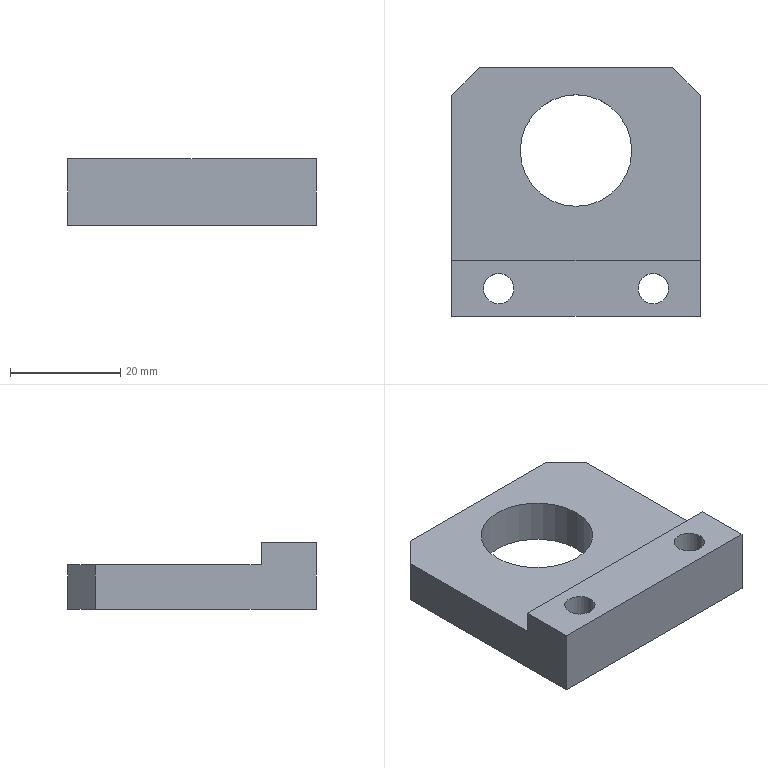Part | STEP file | detection cylinder seat--1 | 1 solid | 16 faces | box 45 x 45 x 12 mm | volume 14666 mm3 | plane 10 | cylinder 6 | commonest cylinder face diameters 5.5 x4 20.2 x2
STEP:
#1=CARTESIAN_POINT('',(0.,0.,0.));
#2=DIRECTION('',(0.,0.,1.));
#3=DIRECTION('',(1.,0.,0.));
#4=AXIS2_PLACEMENT_3D('',#1,#2,#3);
#5=CARTESIAN_POINT('',(11.25,-25.,12.));
#6=VERTEX_POINT('',#5);
#7=CARTESIAN_POINT('',(11.25,-25.,0.));
#8=VERTEX_POINT('',#7);
#9=CARTESIAN_POINT('',(11.25,-25.,12.));
#10=DIRECTION('',(0.,0.,-1.));
#11=VECTOR('',#10,1.);
#12=LINE('',#9,#11);
#13=CARTESIAN_POINT('',(14.,-25.,12.));
#14=DIRECTION('',(0.,0.,-1.));
#15=DIRECTION('',(-1.,0.,0.));
#16=AXIS2_PLACEMENT_3D('',#13,#14,#15);
#17=CYLINDRICAL_SURFACE('',#16,2.75);
#18=CARTESIAN_POINT('',(6.283,0.));
#19=DIRECTION('',(0.,1.));
#20=VECTOR('',#19,1.);
#21=LINE('',#18,#20);
#22=(GEOMETRIC_REPRESENTATION_CONTEXT(2)PARAMETRIC_REPRESENTATION_CONTEXT()REPRESENTATION_CONTEXT('',''));
#23=DEFINITIONAL_REPRESENTATION('',(#21),#22);
#24=PCURVE('',#17,#23);
#25=CARTESIAN_POINT('',(14.,-25.,12.));
#26=DIRECTION('',(0.,0.,-1.));
#27=DIRECTION('',(-1.,0.,0.));
#28=AXIS2_PLACEMENT_3D('',#25,#26,#27);
#29=CYLINDRICAL_SURFACE('',#28,2.75);
#30=CARTESIAN_POINT('',(0.,0.));
#31=DIRECTION('',(0.,1.));
#32=VECTOR('',#31,1.);
#33=LINE('',#30,#32);
#34=(GEOMETRIC_REPRESENTATION_CONTEXT(2)PARAMETRIC_REPRESENTATION_CONTEXT()REPRESENTATION_CONTEXT('',''));
#35=DEFINITIONAL_REPRESENTATION('',(#33),#34);
#36=PCURVE('',#29,#35);
#37=SURFACE_CURVE('',#12,(#24,#36),.PCURVE_S1.);
#38=EDGE_CURVE('',#6,#8,#37,.T.);
#39=ORIENTED_EDGE('',*,*,#38,.T.);
#40=CARTESIAN_POINT('',(16.75,-25.,0.));
#41=VERTEX_POINT('',#40);
#42=CARTESIAN_POINT('',(14.,-25.,0.));
#43=DIRECTION('',(0.,0.,-1.));
#44=DIRECTION('',(-1.,0.,0.));
#45=AXIS2_PLACEMENT_3D('',#42,#43,#44);
#46=CIRCLE('',#45,2.75);
#47=CARTESIAN_POINT('',(0.,12.));
#48=DIRECTION('',(1.,0.));
#49=VECTOR('',#48,1.);
#50=LINE('',#47,#49);
#51=(GEOMETRIC_REPRESENTATION_CONTEXT(2)PARAMETRIC_REPRESENTATION_CONTEXT()REPRESENTATION_CONTEXT('',''));
#52=DEFINITIONAL_REPRESENTATION('',(#50),#51);
#53=PCURVE('',#17,#52);
#54=CARTESIAN_POINT('',(-22.5,-30.,0.));
#55=DIRECTION('',(0.,0.,1.));
#56=DIRECTION('',(1.,0.,0.));
#57=AXIS2_PLACEMENT_3D('',#54,#55,#56);
#58=PLANE('',#57);
#59=CARTESIAN_POINT('',(33.75,5.));
#60=CARTESIAN_POINT('',(33.75,9.763));
#61=CARTESIAN_POINT('',(37.875,7.382));
#62=CARTESIAN_POINT('',(42.,5.));
#63=CARTESIAN_POINT('',(37.875,2.618));
#64=CARTESIAN_POINT('',(33.75,0.2369));
#65=CARTESIAN_POINT('',(33.75,5.));
#66=(BOUNDED_CURVE()B_SPLINE_CURVE(2,(#59,#60,#61,#62,#63,#64,#65),.UNSPECIFIED.,.T.,.F.)B_SPLINE_CURVE_WITH_KNOTS((1,2,2,2,2,1),(-2.094,0.,2.094,4.189,6.283,8.378),.UNSPECIFIED.)CURVE()GEOMETRIC_REPRESENTATION_ITEM()RATIONAL_B_SPLINE_CURVE((1.,0.5,1.,0.5,1.,0.5,1.))REPRESENTATION_ITEM(''));
#67=(GEOMETRIC_REPRESENTATION_CONTEXT(2)PARAMETRIC_REPRESENTATION_CONTEXT()REPRESENTATION_CONTEXT('',''));
#68=DEFINITIONAL_REPRESENTATION('',(#66),#67);
#69=PCURVE('',#58,#68);
#70=SURFACE_CURVE('',#46,(#53,#69),.PCURVE_S1.);
#71=EDGE_CURVE('',#41,#8,#70,.T.);
#72=ORIENTED_EDGE('',*,*,#71,.F.);
#73=CARTESIAN_POINT('',(16.75,-25.,12.));
#74=VERTEX_POINT('',#73);
#75=CARTESIAN_POINT('',(16.75,-25.,12.));
#76=DIRECTION('',(0.,0.,-1.));
#77=VECTOR('',#76,1.);
#78=LINE('',#75,#77);
#79=CARTESIAN_POINT('',(3.142,0.));
#80=DIRECTION('',(0.,1.));
#81=VECTOR('',#80,1.);
#82=LINE('',#79,#81);
#83=(GEOMETRIC_REPRESENTATION_CONTEXT(2)PARAMETRIC_REPRESENTATION_CONTEXT()REPRESENTATION_CONTEXT('',''));
#84=DEFINITIONAL_REPRESENTATION('',(#82),#83);
#85=PCURVE('',#17,#84);
#86=CARTESIAN_POINT('',(3.142,0.));
#87=DIRECTION('',(0.,1.));
#88=VECTOR('',#87,1.);
#89=LINE('',#86,#88);
#90=(GEOMETRIC_REPRESENTATION_CONTEXT(2)PARAMETRIC_REPRESENTATION_CONTEXT()REPRESENTATION_CONTEXT('',''));
#91=DEFINITIONAL_REPRESENTATION('',(#89),#90);
#92=PCURVE('',#29,#91);
#93=SURFACE_CURVE('',#78,(#85,#92),.PCURVE_S1.);
#94=EDGE_CURVE('',#74,#41,#93,.T.);
#95=ORIENTED_EDGE('',*,*,#94,.F.);
#96=CARTESIAN_POINT('',(14.,-25.,12.));
#97=DIRECTION('',(0.,0.,-1.));
#98=DIRECTION('',(-1.,0.,0.));
#99=AXIS2_PLACEMENT_3D('',#96,#97,#98);
#100=CIRCLE('',#99,2.75);
#101=CARTESIAN_POINT('',(0.,0.));
#102=DIRECTION('',(1.,0.));
#103=VECTOR('',#102,1.);
#104=LINE('',#101,#103);
#105=(GEOMETRIC_REPRESENTATION_CONTEXT(2)PARAMETRIC_REPRESENTATION_CONTEXT()REPRESENTATION_CONTEXT('',''));
#106=DEFINITIONAL_REPRESENTATION('',(#104),#105);
#107=PCURVE('',#17,#106);
#108=CARTESIAN_POINT('',(-22.5,-30.,12.));
#109=DIRECTION('',(0.,0.,1.));
#110=DIRECTION('',(1.,0.,0.));
#111=AXIS2_PLACEMENT_3D('',#108,#109,#110);
#112=PLANE('',#111);
#113=CARTESIAN_POINT('',(33.75,5.));
#114=CARTESIAN_POINT('',(33.75,9.763));
#115=CARTESIAN_POINT('',(37.875,7.382));
#116=CARTESIAN_POINT('',(42.,5.));
#117=CARTESIAN_POINT('',(37.875,2.618));
#118=CARTESIAN_POINT('',(33.75,0.2369));
#119=CARTESIAN_POINT('',(33.75,5.));
#120=(BOUNDED_CURVE()B_SPLINE_CURVE(2,(#113,#114,#115,#116,#117,#118,#119),.UNSPECIFIED.,.T.,.F.)B_SPLINE_CURVE_WITH_KNOTS((1,2,2,2,2,1),(-2.094,0.,2.094,4.189,6.283,8.378),.UNSPECIFIED.)CURVE()GEOMETRIC_REPRESENTATION_ITEM()RATIONAL_B_SPLINE_CURVE((1.,0.5,1.,0.5,1.,0.5,1.))REPRESENTATION_ITEM(''));
#121=(GEOMETRIC_REPRESENTATION_CONTEXT(2)PARAMETRIC_REPRESENTATION_CONTEXT()REPRESENTATION_CONTEXT('',''));
#122=DEFINITIONAL_REPRESENTATION('',(#120),#121);
#123=PCURVE('',#112,#122);
#124=SURFACE_CURVE('',#100,(#107,#123),.PCURVE_S1.);
#125=EDGE_CURVE('',#74,#6,#124,.T.);
#126=ORIENTED_EDGE('',*,*,#125,.T.);
#127=EDGE_LOOP('',(#39,#72,#95,#126));
#128=FACE_BOUND('',#127,.F.);
#129=ADVANCED_FACE('',(#128),#17,.F.);
#130=CARTESIAN_POINT('',(-16.75,-25.,12.));
#131=VERTEX_POINT('',#130);
#132=CARTESIAN_POINT('',(-16.75,-25.,0.));
#133=VERTEX_POINT('',#132);
#134=CARTESIAN_POINT('',(-16.75,-25.,12.));
#135=DIRECTION('',(0.,0.,-1.));
#136=VECTOR('',#135,1.);
#137=LINE('',#134,#136);
#138=CARTESIAN_POINT('',(-14.,-25.,12.));
#139=DIRECTION('',(0.,0.,-1.));
#140=DIRECTION('',(-1.,0.,0.));
#141=AXIS2_PLACEMENT_3D('',#138,#139,#140);
#142=CYLINDRICAL_SURFACE('',#141,2.75);
#143=CARTESIAN_POINT('',(6.283,0.));
#144=DIRECTION('',(0.,1.));
#145=VECTOR('',#144,1.);
#146=LINE('',#143,#145);
#147=(GEOMETRIC_REPRESENTATION_CONTEXT(2)PARAMETRIC_REPRESENTATION_CONTEXT()REPRESENTATION_CONTEXT('',''));
#148=DEFINITIONAL_REPRESENTATION('',(#146),#147);
#149=PCURVE('',#142,#148);
#150=CARTESIAN_POINT('',(-14.,-25.,12.));
#151=DIRECTION('',(0.,0.,-1.));
#152=DIRECTION('',(-1.,0.,0.));
#153=AXIS2_PLACEMENT_3D('',#150,#151,#152);
#154=CYLINDRICAL_SURFACE('',#153,2.75);
#155=CARTESIAN_POINT('',(0.,0.));
#156=DIRECTION('',(0.,1.));
#157=VECTOR('',#156,1.);
#158=LINE('',#155,#157);
#159=(GEOMETRIC_REPRESENTATION_CONTEXT(2)PARAMETRIC_REPRESENTATION_CONTEXT()REPRESENTATION_CONTEXT('',''));
#160=DEFINITIONAL_REPRESENTATION('',(#158),#159);
#161=PCURVE('',#154,#160);
#162=SURFACE_CURVE('',#137,(#149,#161),.PCURVE_S1.);
#163=EDGE_CURVE('',#131,#133,#162,.T.);
#164=ORIENTED_EDGE('',*,*,#163,.T.);
#165=CARTESIAN_POINT('',(-11.25,-25.,0.));
#166=VERTEX_POINT('',#165);
#167=CARTESIAN_POINT('',(-14.,-25.,0.));
#168=DIRECTION('',(0.,0.,-1.));
#169=DIRECTION('',(-1.,0.,0.));
#170=AXIS2_PLACEMENT_3D('',#167,#168,#169);
#171=CIRCLE('',#170,2.75);
#172=CARTESIAN_POINT('',(0.,12.));
#173=DIRECTION('',(1.,0.));
#174=VECTOR('',#173,1.);
#175=LINE('',#172,#174);
#176=(GEOMETRIC_REPRESENTATION_CONTEXT(2)PARAMETRIC_REPRESENTATION_CONTEXT()REPRESENTATION_CONTEXT('',''));
#177=DEFINITIONAL_REPRESENTATION('',(#175),#176);
#178=PCURVE('',#142,#177);
#179=CARTESIAN_POINT('',(5.75,5.));
#180=CARTESIAN_POINT('',(5.75,9.763));
#181=CARTESIAN_POINT('',(9.875,7.382));
#182=CARTESIAN_POINT('',(14.,5.));
#183=CARTESIAN_POINT('',(9.875,2.618));
#184=CARTESIAN_POINT('',(5.75,0.2369));
#185=CARTESIAN_POINT('',(5.75,5.));
#186=(BOUNDED_CURVE()B_SPLINE_CURVE(2,(#179,#180,#181,#182,#183,#184,#185),.UNSPECIFIED.,.T.,.F.)B_SPLINE_CURVE_WITH_KNOTS((1,2,2,2,2,1),(-2.094,0.,2.094,4.189,6.283,8.378),.UNSPECIFIED.)CURVE()GEOMETRIC_REPRESENTATION_ITEM()RATIONAL_B_SPLINE_CURVE((1.,0.5,1.,0.5,1.,0.5,1.))REPRESENTATION_ITEM(''));
#187=(GEOMETRIC_REPRESENTATION_CONTEXT(2)PARAMETRIC_REPRESENTATION_CONTEXT()REPRESENTATION_CONTEXT('',''));
#188=DEFINITIONAL_REPRESENTATION('',(#186),#187);
#189=PCURVE('',#58,#188);
#190=SURFACE_CURVE('',#171,(#178,#189),.PCURVE_S1.);
#191=EDGE_CURVE('',#166,#133,#190,.T.);
#192=ORIENTED_EDGE('',*,*,#191,.F.);
#193=CARTESIAN_POINT('',(-11.25,-25.,12.));
#194=VERTEX_POINT('',#193);
#195=CARTESIAN_POINT('',(-11.25,-25.,12.));
#196=DIRECTION('',(0.,0.,-1.));
#197=VECTOR('',#196,1.);
#198=LINE('',#195,#197);
#199=CARTESIAN_POINT('',(3.142,0.));
#200=DIRECTION('',(0.,1.));
#201=VECTOR('',#200,1.);
#202=LINE('',#199,#201);
#203=(GEOMETRIC_REPRESENTATION_CONTEXT(2)PARAMETRIC_REPRESENTATION_CONTEXT()REPRESENTATION_CONTEXT('',''));
#204=DEFINITIONAL_REPRESENTATION('',(#202),#203);
#205=PCURVE('',#142,#204);
#206=CARTESIAN_POINT('',(3.142,0.));
#207=DIRECTION('',(0.,1.));
#208=VECTOR('',#207,1.);
#209=LINE('',#206,#208);
#210=(GEOMETRIC_REPRESENTATION_CONTEXT(2)PARAMETRIC_REPRESENTATION_CONTEXT()REPRESENTATION_CONTEXT('',''));
#211=DEFINITIONAL_REPRESENTATION('',(#209),#210);
#212=PCURVE('',#154,#211);
#213=SURFACE_CURVE('',#198,(#205,#212),.PCURVE_S1.);
#214=EDGE_CURVE('',#194,#166,#213,.T.);
#215=ORIENTED_EDGE('',*,*,#214,.F.);
#216=CARTESIAN_POINT('',(-14.,-25.,12.));
#217=DIRECTION('',(0.,0.,-1.));
#218=DIRECTION('',(-1.,0.,0.));
#219=AXIS2_PLACEMENT_3D('',#216,#217,#218);
#220=CIRCLE('',#219,2.75);
#221=CARTESIAN_POINT('',(0.,0.));
#222=DIRECTION('',(1.,0.));
#223=VECTOR('',#222,1.);
#224=LINE('',#221,#223);
#225=(GEOMETRIC_REPRESENTATION_CONTEXT(2)PARAMETRIC_REPRESENTATION_CONTEXT()REPRESENTATION_CONTEXT('',''));
#226=DEFINITIONAL_REPRESENTATION('',(#224),#225);
#227=PCURVE('',#142,#226);
#228=CARTESIAN_POINT('',(5.75,5.));
#229=CARTESIAN_POINT('',(5.75,9.763));
#230=CARTESIAN_POINT('',(9.875,7.382));
#231=CARTESIAN_POINT('',(14.,5.));
#232=CARTESIAN_POINT('',(9.875,2.618));
#233=CARTESIAN_POINT('',(5.75,0.2369));
#234=CARTESIAN_POINT('',(5.75,5.));
#235=(BOUNDED_CURVE()B_SPLINE_CURVE(2,(#228,#229,#230,#231,#232,#233,#234),.UNSPECIFIED.,.T.,.F.)B_SPLINE_CURVE_WITH_KNOTS((1,2,2,2,2,1),(-2.094,0.,2.094,4.189,6.283,8.378),.UNSPECIFIED.)CURVE()GEOMETRIC_REPRESENTATION_ITEM()RATIONAL_B_SPLINE_CURVE((1.,0.5,1.,0.5,1.,0.5,1.))REPRESENTATION_ITEM(''));
#236=(GEOMETRIC_REPRESENTATION_CONTEXT(2)PARAMETRIC_REPRESENTATION_CONTEXT()REPRESENTATION_CONTEXT('',''));
#237=DEFINITIONAL_REPRESENTATION('',(#235),#236);
#238=PCURVE('',#112,#237);
#239=SURFACE_CURVE('',#220,(#227,#238),.PCURVE_S1.);
#240=EDGE_CURVE('',#194,#131,#239,.T.);
#241=ORIENTED_EDGE('',*,*,#240,.T.);
#242=EDGE_LOOP('',(#164,#192,#215,#241));
#243=FACE_BOUND('',#242,.F.);
#244=ADVANCED_FACE('',(#243),#142,.F.);
#245=CARTESIAN_POINT('',(-10.1,0.,8.));
#246=VERTEX_POINT('',#245);
#247=CARTESIAN_POINT('',(-10.1,0.,0.));
#248=VERTEX_POINT('',#247);
#249=CARTESIAN_POINT('',(-10.1,0.,12.));
#250=DIRECTION('',(0.,0.,-1.));
#251=VECTOR('',#250,1.);
#252=LINE('',#249,#251);
#253=CARTESIAN_POINT('',(0.,0.,12.));
#254=DIRECTION('',(0.,0.,-1.));
#255=DIRECTION('',(-1.,0.,0.));
#256=AXIS2_PLACEMENT_3D('',#253,#254,#255);
#257=CYLINDRICAL_SURFACE('',#256,10.1);
#258=CARTESIAN_POINT('',(6.283,0.));
#259=DIRECTION('',(0.,1.));
#260=VECTOR('',#259,1.);
#261=LINE('',#258,#260);
#262=(GEOMETRIC_REPRESENTATION_CONTEXT(2)PARAMETRIC_REPRESENTATION_CONTEXT()REPRESENTATION_CONTEXT('',''));
#263=DEFINITIONAL_REPRESENTATION('',(#261),#262);
#264=PCURVE('',#257,#263);
#265=CARTESIAN_POINT('',(0.,0.,12.));
#266=DIRECTION('',(0.,0.,-1.));
#267=DIRECTION('',(-1.,0.,0.));
#268=AXIS2_PLACEMENT_3D('',#265,#266,#267);
#269=CYLINDRICAL_SURFACE('',#268,10.1);
#270=CARTESIAN_POINT('',(0.,0.));
#271=DIRECTION('',(0.,1.));
#272=VECTOR('',#271,1.);
#273=LINE('',#270,#272);
#274=(GEOMETRIC_REPRESENTATION_CONTEXT(2)PARAMETRIC_REPRESENTATION_CONTEXT()REPRESENTATION_CONTEXT('',''));
#275=DEFINITIONAL_REPRESENTATION('',(#273),#274);
#276=PCURVE('',#269,#275);
#277=SURFACE_CURVE('',#252,(#264,#276),.PCURVE_S1.);
#278=EDGE_CURVE('',#246,#248,#277,.T.);
#279=ORIENTED_EDGE('',*,*,#278,.T.);
#280=CARTESIAN_POINT('',(10.1,0.,0.));
#281=VERTEX_POINT('',#280);
#282=CARTESIAN_POINT('',(0.,0.,0.));
#283=DIRECTION('',(0.,0.,1.));
#284=DIRECTION('',(1.,0.,0.));
#285=AXIS2_PLACEMENT_3D('',#282,#283,#284);
#286=CIRCLE('',#285,10.1);
#287=CARTESIAN_POINT('',(9.425,12.));
#288=DIRECTION('',(-1.,0.));
#289=VECTOR('',#288,1.);
#290=LINE('',#287,#289);
#291=(GEOMETRIC_REPRESENTATION_CONTEXT(2)PARAMETRIC_REPRESENTATION_CONTEXT()REPRESENTATION_CONTEXT('',''));
#292=DEFINITIONAL_REPRESENTATION('',(#290),#291);
#293=PCURVE('',#257,#292);
#294=CARTESIAN_POINT('',(22.5,30.));
#295=DIRECTION('',(1.,0.));
#296=AXIS2_PLACEMENT_2D('',#294,#295);
#297=CIRCLE('',#296,10.1);
#298=(GEOMETRIC_REPRESENTATION_CONTEXT(2)PARAMETRIC_REPRESENTATION_CONTEXT()REPRESENTATION_CONTEXT('',''));
#299=DEFINITIONAL_REPRESENTATION('',(#297),#298);
#300=PCURVE('',#58,#299);
#301=SURFACE_CURVE('',#286,(#293,#300),.PCURVE_S1.);
#302=EDGE_CURVE('',#248,#281,#301,.T.);
#303=ORIENTED_EDGE('',*,*,#302,.T.);
#304=CARTESIAN_POINT('',(10.1,0.,8.));
#305=VERTEX_POINT('',#304);
#306=CARTESIAN_POINT('',(10.1,0.,12.));
#307=DIRECTION('',(0.,0.,-1.));
#308=VECTOR('',#307,1.);
#309=LINE('',#306,#308);
#310=CARTESIAN_POINT('',(3.142,0.));
#311=DIRECTION('',(0.,1.));
#312=VECTOR('',#311,1.);
#313=LINE('',#310,#312);
#314=(GEOMETRIC_REPRESENTATION_CONTEXT(2)PARAMETRIC_REPRESENTATION_CONTEXT()REPRESENTATION_CONTEXT('',''));
#315=DEFINITIONAL_REPRESENTATION('',(#313),#314);
#316=PCURVE('',#257,#315);
#317=CARTESIAN_POINT('',(3.142,0.));
#318=DIRECTION('',(0.,1.));
#319=VECTOR('',#318,1.);
#320=LINE('',#317,#319);
#321=(GEOMETRIC_REPRESENTATION_CONTEXT(2)PARAMETRIC_REPRESENTATION_CONTEXT()REPRESENTATION_CONTEXT('',''));
#322=DEFINITIONAL_REPRESENTATION('',(#320),#321);
#323=PCURVE('',#269,#322);
#324=SURFACE_CURVE('',#309,(#316,#323),.PCURVE_S1.);
#325=EDGE_CURVE('',#305,#281,#324,.T.);
#326=ORIENTED_EDGE('',*,*,#325,.F.);
#327=CARTESIAN_POINT('',(0.,0.,8.));
#328=DIRECTION('',(0.,0.,1.));
#329=DIRECTION('',(1.,0.,0.));
#330=AXIS2_PLACEMENT_3D('',#327,#328,#329);
#331=CIRCLE('',#330,10.1);
#332=CARTESIAN_POINT('',(9.425,4.));
#333=DIRECTION('',(-1.,0.));
#334=VECTOR('',#333,1.);
#335=LINE('',#332,#334);
#336=(GEOMETRIC_REPRESENTATION_CONTEXT(2)PARAMETRIC_REPRESENTATION_CONTEXT()REPRESENTATION_CONTEXT('',''));
#337=DEFINITIONAL_REPRESENTATION('',(#335),#336);
#338=PCURVE('',#257,#337);
#339=CARTESIAN_POINT('',(-34.163,-20.,8.));
#340=DIRECTION('',(0.,0.,1.));
#341=DIRECTION('',(1.,0.,0.));
#342=AXIS2_PLACEMENT_3D('',#339,#340,#341);
#343=PLANE('',#342);
#344=CARTESIAN_POINT('',(34.163,20.));
#345=DIRECTION('',(1.,0.));
#346=AXIS2_PLACEMENT_2D('',#344,#345);
#347=CIRCLE('',#346,10.1);
#348=(GEOMETRIC_REPRESENTATION_CONTEXT(2)PARAMETRIC_REPRESENTATION_CONTEXT()REPRESENTATION_CONTEXT('',''));
#349=DEFINITIONAL_REPRESENTATION('',(#347),#348);
#350=PCURVE('',#343,#349);
#351=SURFACE_CURVE('',#331,(#338,#350),.PCURVE_S1.);
#352=EDGE_CURVE('',#246,#305,#351,.T.);
#353=ORIENTED_EDGE('',*,*,#352,.F.);
#354=EDGE_LOOP('',(#279,#303,#326,#353));
#355=FACE_BOUND('',#354,.F.);
#356=ADVANCED_FACE('',(#355),#257,.F.);
#357=CARTESIAN_POINT('',(17.5,15.,8.));
#358=VERTEX_POINT('',#357);
#359=CARTESIAN_POINT('',(-17.5,15.,8.));
#360=VERTEX_POINT('',#359);
#361=CARTESIAN_POINT('',(-22.5,15.,8.));
#362=DIRECTION('',(-1.,0.,0.));
#363=VECTOR('',#362,1.);
#364=LINE('',#361,#363);
#365=CARTESIAN_POINT('',(-22.5,15.,12.));
#366=DIRECTION('',(0.,-1.,0.));
#367=DIRECTION('',(0.,0.,-1.));
#368=AXIS2_PLACEMENT_3D('',#365,#366,#367);
#369=PLANE('',#368);
#370=CARTESIAN_POINT('',(4.,0.));
#371=DIRECTION('',(0.,-1.));
#372=VECTOR('',#371,1.);
#373=LINE('',#370,#372);
#374=(GEOMETRIC_REPRESENTATION_CONTEXT(2)PARAMETRIC_REPRESENTATION_CONTEXT()REPRESENTATION_CONTEXT('',''));
#375=DEFINITIONAL_REPRESENTATION('',(#373),#374);
#376=PCURVE('',#369,#375);
#377=CARTESIAN_POINT('',(11.663,35.));
#378=DIRECTION('',(-1.,0.));
#379=VECTOR('',#378,1.);
#380=LINE('',#377,#379);
#381=(GEOMETRIC_REPRESENTATION_CONTEXT(2)PARAMETRIC_REPRESENTATION_CONTEXT()REPRESENTATION_CONTEXT('',''));
#382=DEFINITIONAL_REPRESENTATION('',(#380),#381);
#383=PCURVE('',#343,#382);
#384=SURFACE_CURVE('',#364,(#376,#383),.PCURVE_S1.);
#385=EDGE_CURVE('',#358,#360,#384,.T.);
#386=ORIENTED_EDGE('',*,*,#385,.F.);
#387=CARTESIAN_POINT('',(17.5,15.,0.));
#388=VERTEX_POINT('',#387);
#389=CARTESIAN_POINT('',(17.5,15.,12.));
#390=DIRECTION('',(0.,0.,-1.));
#391=VECTOR('',#390,1.);
#392=LINE('',#389,#391);
#393=CARTESIAN_POINT('',(0.,40.));
#394=DIRECTION('',(1.,0.));
#395=VECTOR('',#394,1.);
#396=LINE('',#393,#395);
#397=(GEOMETRIC_REPRESENTATION_CONTEXT(2)PARAMETRIC_REPRESENTATION_CONTEXT()REPRESENTATION_CONTEXT('',''));
#398=DEFINITIONAL_REPRESENTATION('',(#396),#397);
#399=PCURVE('',#369,#398);
#400=CARTESIAN_POINT('',(17.5,15.,12.));
#401=DIRECTION('',(-0.7071,-0.7071,0.));
#402=DIRECTION('',(0.7071,-0.7071,0.));
#403=AXIS2_PLACEMENT_3D('',#400,#401,#402);
#404=PLANE('',#403);
#405=CARTESIAN_POINT('',(0.,0.));
#406=DIRECTION('',(0.,-1.));
#407=VECTOR('',#406,1.);
#408=LINE('',#405,#407);
#409=(GEOMETRIC_REPRESENTATION_CONTEXT(2)PARAMETRIC_REPRESENTATION_CONTEXT()REPRESENTATION_CONTEXT('',''));
#410=DEFINITIONAL_REPRESENTATION('',(#408),#409);
#411=PCURVE('',#404,#410);
#412=SURFACE_CURVE('',#392,(#399,#411),.PCURVE_S1.);
#413=EDGE_CURVE('',#358,#388,#412,.T.);
#414=ORIENTED_EDGE('',*,*,#413,.T.);
#415=CARTESIAN_POINT('',(-17.5,15.,0.));
#416=VERTEX_POINT('',#415);
#417=CARTESIAN_POINT('',(-22.5,15.,0.));
#418=DIRECTION('',(-1.,0.,0.));
#419=VECTOR('',#418,1.);
#420=LINE('',#417,#419);
#421=CARTESIAN_POINT('',(12.,0.));
#422=DIRECTION('',(0.,-1.));
#423=VECTOR('',#422,1.);
#424=LINE('',#421,#423);
#425=(GEOMETRIC_REPRESENTATION_CONTEXT(2)PARAMETRIC_REPRESENTATION_CONTEXT()REPRESENTATION_CONTEXT('',''));
#426=DEFINITIONAL_REPRESENTATION('',(#424),#425);
#427=PCURVE('',#369,#426);
#428=CARTESIAN_POINT('',(0.,45.));
#429=DIRECTION('',(-1.,0.));
#430=VECTOR('',#429,1.);
#431=LINE('',#428,#430);
#432=(GEOMETRIC_REPRESENTATION_CONTEXT(2)PARAMETRIC_REPRESENTATION_CONTEXT()REPRESENTATION_CONTEXT('',''));
#433=DEFINITIONAL_REPRESENTATION('',(#431),#432);
#434=PCURVE('',#58,#433);
#435=SURFACE_CURVE('',#420,(#427,#434),.PCURVE_S1.);
#436=EDGE_CURVE('',#388,#416,#435,.T.);
#437=ORIENTED_EDGE('',*,*,#436,.T.);
#438=CARTESIAN_POINT('',(-17.5,15.,12.));
#439=DIRECTION('',(0.,0.,1.));
#440=VECTOR('',#439,1.);
#441=LINE('',#438,#440);
#442=CARTESIAN_POINT('',(0.,5.));
#443=DIRECTION('',(-1.,0.));
#444=VECTOR('',#443,1.);
#445=LINE('',#442,#444);
#446=(GEOMETRIC_REPRESENTATION_CONTEXT(2)PARAMETRIC_REPRESENTATION_CONTEXT()REPRESENTATION_CONTEXT('',''));
#447=DEFINITIONAL_REPRESENTATION('',(#445),#446);
#448=PCURVE('',#369,#447);
#449=CARTESIAN_POINT('',(-22.5,10.,12.));
#450=DIRECTION('',(0.7071,-0.7071,0.));
#451=DIRECTION('',(0.7071,0.7071,0.));
#452=AXIS2_PLACEMENT_3D('',#449,#450,#451);
#453=PLANE('',#452);
#454=CARTESIAN_POINT('',(7.071,0.));
#455=DIRECTION('',(0.,1.));
#456=VECTOR('',#455,1.);
#457=LINE('',#454,#456);
#458=(GEOMETRIC_REPRESENTATION_CONTEXT(2)PARAMETRIC_REPRESENTATION_CONTEXT()REPRESENTATION_CONTEXT('',''));
#459=DEFINITIONAL_REPRESENTATION('',(#457),#458);
#460=PCURVE('',#453,#459);
#461=SURFACE_CURVE('',#441,(#448,#460),.PCURVE_S1.);
#462=EDGE_CURVE('',#416,#360,#461,.T.);
#463=ORIENTED_EDGE('',*,*,#462,.T.);
#464=EDGE_LOOP('',(#386,#414,#437,#463));
#465=FACE_BOUND('',#464,.T.);
#466=ADVANCED_FACE('',(#465),#369,.F.);
#467=CARTESIAN_POINT('',(0.,0.,0.));
#468=DIRECTION('',(0.,0.,1.));
#469=DIRECTION('',(1.,0.,0.));
#470=AXIS2_PLACEMENT_3D('',#467,#468,#469);
#471=CIRCLE('',#470,10.1);
#472=CARTESIAN_POINT('',(3.142,12.));
#473=DIRECTION('',(-1.,0.));
#474=VECTOR('',#473,1.);
#475=LINE('',#472,#474);
#476=(GEOMETRIC_REPRESENTATION_CONTEXT(2)PARAMETRIC_REPRESENTATION_CONTEXT()REPRESENTATION_CONTEXT('',''));
#477=DEFINITIONAL_REPRESENTATION('',(#475),#476);
#478=PCURVE('',#269,#477);
#479=CARTESIAN_POINT('',(22.5,30.));
#480=DIRECTION('',(1.,0.));
#481=AXIS2_PLACEMENT_2D('',#479,#480);
#482=CIRCLE('',#481,10.1);
#483=(GEOMETRIC_REPRESENTATION_CONTEXT(2)PARAMETRIC_REPRESENTATION_CONTEXT()REPRESENTATION_CONTEXT('',''));
#484=DEFINITIONAL_REPRESENTATION('',(#482),#483);
#485=PCURVE('',#58,#484);
#486=SURFACE_CURVE('',#471,(#478,#485),.PCURVE_S1.);
#487=EDGE_CURVE('',#281,#248,#486,.T.);
#488=ORIENTED_EDGE('',*,*,#487,.T.);
#489=ORIENTED_EDGE('',*,*,#278,.F.);
#490=CARTESIAN_POINT('',(0.,0.,8.));
#491=DIRECTION('',(0.,0.,1.));
#492=DIRECTION('',(1.,0.,0.));
#493=AXIS2_PLACEMENT_3D('',#490,#491,#492);
#494=CIRCLE('',#493,10.1);
#495=CARTESIAN_POINT('',(3.142,4.));
#496=DIRECTION('',(-1.,0.));
#497=VECTOR('',#496,1.);
#498=LINE('',#495,#497);
#499=(GEOMETRIC_REPRESENTATION_CONTEXT(2)PARAMETRIC_REPRESENTATION_CONTEXT()REPRESENTATION_CONTEXT('',''));
#500=DEFINITIONAL_REPRESENTATION('',(#498),#499);
#501=PCURVE('',#269,#500);
#502=CARTESIAN_POINT('',(34.163,20.));
#503=DIRECTION('',(1.,0.));
#504=AXIS2_PLACEMENT_2D('',#502,#503);
#505=CIRCLE('',#504,10.1);
#506=(GEOMETRIC_REPRESENTATION_CONTEXT(2)PARAMETRIC_REPRESENTATION_CONTEXT()REPRESENTATION_CONTEXT('',''));
#507=DEFINITIONAL_REPRESENTATION('',(#505),#506);
#508=PCURVE('',#343,#507);
#509=SURFACE_CURVE('',#494,(#501,#508),.PCURVE_S1.);
#510=EDGE_CURVE('',#305,#246,#509,.T.);
#511=ORIENTED_EDGE('',*,*,#510,.F.);
#512=ORIENTED_EDGE('',*,*,#325,.T.);
#513=EDGE_LOOP('',(#488,#489,#511,#512));
#514=FACE_BOUND('',#513,.F.);
#515=ADVANCED_FACE('',(#514),#269,.F.);
#516=CARTESIAN_POINT('',(-22.5,10.,8.));
#517=VERTEX_POINT('',#516);
#518=CARTESIAN_POINT('',(-22.5,10.,0.));
#519=VERTEX_POINT('',#518);
#520=CARTESIAN_POINT('',(-22.5,10.,12.));
#521=DIRECTION('',(0.,0.,-1.));
#522=VECTOR('',#521,1.);
#523=LINE('',#520,#522);
#524=CARTESIAN_POINT('',(0.,0.));
#525=DIRECTION('',(0.,-1.));
#526=VECTOR('',#525,1.);
#527=LINE('',#524,#526);
#528=(GEOMETRIC_REPRESENTATION_CONTEXT(2)PARAMETRIC_REPRESENTATION_CONTEXT()REPRESENTATION_CONTEXT('',''));
#529=DEFINITIONAL_REPRESENTATION('',(#527),#528);
#530=PCURVE('',#453,#529);
#531=CARTESIAN_POINT('',(-22.5,15.,12.));
#532=DIRECTION('',(1.,0.,0.));
#533=DIRECTION('',(0.,1.,0.));
#534=AXIS2_PLACEMENT_3D('',#531,#532,#533);
#535=PLANE('',#534);
#536=CARTESIAN_POINT('',(-5.,0.));
#537=DIRECTION('',(0.,-1.));
#538=VECTOR('',#537,1.);
#539=LINE('',#536,#538);
#540=(GEOMETRIC_REPRESENTATION_CONTEXT(2)PARAMETRIC_REPRESENTATION_CONTEXT()REPRESENTATION_CONTEXT('',''));
#541=DEFINITIONAL_REPRESENTATION('',(#539),#540);
#542=PCURVE('',#535,#541);
#543=SURFACE_CURVE('',#523,(#530,#542),.PCURVE_S1.);
#544=EDGE_CURVE('',#517,#519,#543,.T.);
#545=ORIENTED_EDGE('',*,*,#544,.F.);
#546=CARTESIAN_POINT('',(-22.5,10.,8.));
#547=DIRECTION('',(0.7071,0.7071,0.));
#548=VECTOR('',#547,1.);
#549=LINE('',#546,#548);
#550=CARTESIAN_POINT('',(0.,-4.));
#551=DIRECTION('',(1.,0.));
#552=VECTOR('',#551,1.);
#553=LINE('',#550,#552);
#554=(GEOMETRIC_REPRESENTATION_CONTEXT(2)PARAMETRIC_REPRESENTATION_CONTEXT()REPRESENTATION_CONTEXT('',''));
#555=DEFINITIONAL_REPRESENTATION('',(#553),#554);
#556=PCURVE('',#453,#555);
#557=CARTESIAN_POINT('',(11.663,30.));
#558=DIRECTION('',(0.7071,0.7071));
#559=VECTOR('',#558,1.);
#560=LINE('',#557,#559);
#561=(GEOMETRIC_REPRESENTATION_CONTEXT(2)PARAMETRIC_REPRESENTATION_CONTEXT()REPRESENTATION_CONTEXT('',''));
#562=DEFINITIONAL_REPRESENTATION('',(#560),#561);
#563=PCURVE('',#343,#562);
#564=SURFACE_CURVE('',#549,(#556,#563),.PCURVE_S1.);
#565=EDGE_CURVE('',#517,#360,#564,.T.);
#566=ORIENTED_EDGE('',*,*,#565,.T.);
#567=ORIENTED_EDGE('',*,*,#462,.F.);
#568=CARTESIAN_POINT('',(-22.5,10.,0.));
#569=DIRECTION('',(0.7071,0.7071,0.));
#570=VECTOR('',#569,1.);
#571=LINE('',#568,#570);
#572=CARTESIAN_POINT('',(0.,-12.));
#573=DIRECTION('',(1.,0.));
#574=VECTOR('',#573,1.);
#575=LINE('',#572,#574);
#576=(GEOMETRIC_REPRESENTATION_CONTEXT(2)PARAMETRIC_REPRESENTATION_CONTEXT()REPRESENTATION_CONTEXT('',''));
#577=DEFINITIONAL_REPRESENTATION('',(#575),#576);
#578=PCURVE('',#453,#577);
#579=CARTESIAN_POINT('',(0.,40.));
#580=DIRECTION('',(0.7071,0.7071));
#581=VECTOR('',#580,1.);
#582=LINE('',#579,#581);
#583=(GEOMETRIC_REPRESENTATION_CONTEXT(2)PARAMETRIC_REPRESENTATION_CONTEXT()REPRESENTATION_CONTEXT('',''));
#584=DEFINITIONAL_REPRESENTATION('',(#582),#583);
#585=PCURVE('',#58,#584);
#586=SURFACE_CURVE('',#571,(#578,#585),.PCURVE_S1.);
#587=EDGE_CURVE('',#519,#416,#586,.T.);
#588=ORIENTED_EDGE('',*,*,#587,.F.);
#589=EDGE_LOOP('',(#545,#566,#567,#588));
#590=FACE_BOUND('',#589,.T.);
#591=ADVANCED_FACE('',(#590),#453,.F.);
#592=ORIENTED_EDGE('',*,*,#413,.F.);
#593=CARTESIAN_POINT('',(22.5,10.,8.));
#594=VERTEX_POINT('',#593);
#595=CARTESIAN_POINT('',(17.5,15.,8.));
#596=DIRECTION('',(0.7071,-0.7071,0.));
#597=VECTOR('',#596,1.);
#598=LINE('',#595,#597);
#599=CARTESIAN_POINT('',(0.,-4.));
#600=DIRECTION('',(1.,0.));
#601=VECTOR('',#600,1.);
#602=LINE('',#599,#601);
#603=(GEOMETRIC_REPRESENTATION_CONTEXT(2)PARAMETRIC_REPRESENTATION_CONTEXT()REPRESENTATION_CONTEXT('',''));
#604=DEFINITIONAL_REPRESENTATION('',(#602),#603);
#605=PCURVE('',#404,#604);
#606=CARTESIAN_POINT('',(51.663,35.));
#607=DIRECTION('',(0.7071,-0.7071));
#608=VECTOR('',#607,1.);
#609=LINE('',#606,#608);
#610=(GEOMETRIC_REPRESENTATION_CONTEXT(2)PARAMETRIC_REPRESENTATION_CONTEXT()REPRESENTATION_CONTEXT('',''));
#611=DEFINITIONAL_REPRESENTATION('',(#609),#610);
#612=PCURVE('',#343,#611);
#613=SURFACE_CURVE('',#598,(#605,#612),.PCURVE_S1.);
#614=EDGE_CURVE('',#358,#594,#613,.T.);
#615=ORIENTED_EDGE('',*,*,#614,.T.);
#616=CARTESIAN_POINT('',(22.5,10.,0.));
#617=VERTEX_POINT('',#616);
#618=CARTESIAN_POINT('',(22.5,10.,12.));
#619=DIRECTION('',(0.,0.,1.));
#620=VECTOR('',#619,1.);
#621=LINE('',#618,#620);
#622=CARTESIAN_POINT('',(7.071,0.));
#623=DIRECTION('',(0.,1.));
#624=VECTOR('',#623,1.);
#625=LINE('',#622,#624);
#626=(GEOMETRIC_REPRESENTATION_CONTEXT(2)PARAMETRIC_REPRESENTATION_CONTEXT()REPRESENTATION_CONTEXT('',''));
#627=DEFINITIONAL_REPRESENTATION('',(#625),#626);
#628=PCURVE('',#404,#627);
#629=CARTESIAN_POINT('',(22.5,15.,12.));
#630=DIRECTION('',(-1.,0.,0.));
#631=DIRECTION('',(0.,-1.,0.));
#632=AXIS2_PLACEMENT_3D('',#629,#630,#631);
#633=PLANE('',#632);
#634=CARTESIAN_POINT('',(5.,0.));
#635=DIRECTION('',(0.,1.));
#636=VECTOR('',#635,1.);
#637=LINE('',#634,#636);
#638=(GEOMETRIC_REPRESENTATION_CONTEXT(2)PARAMETRIC_REPRESENTATION_CONTEXT()REPRESENTATION_CONTEXT('',''));
#639=DEFINITIONAL_REPRESENTATION('',(#637),#638);
#640=PCURVE('',#633,#639);
#641=SURFACE_CURVE('',#621,(#628,#640),.PCURVE_S1.);
#642=EDGE_CURVE('',#617,#594,#641,.T.);
#643=ORIENTED_EDGE('',*,*,#642,.F.);
#644=CARTESIAN_POINT('',(17.5,15.,0.));
#645=DIRECTION('',(0.7071,-0.7071,0.));
#646=VECTOR('',#645,1.);
#647=LINE('',#644,#646);
#648=CARTESIAN_POINT('',(0.,-12.));
#649=DIRECTION('',(1.,0.));
#650=VECTOR('',#649,1.);
#651=LINE('',#648,#650);
#652=(GEOMETRIC_REPRESENTATION_CONTEXT(2)PARAMETRIC_REPRESENTATION_CONTEXT()REPRESENTATION_CONTEXT('',''));
#653=DEFINITIONAL_REPRESENTATION('',(#651),#652);
#654=PCURVE('',#404,#653);
#655=CARTESIAN_POINT('',(40.,45.));
#656=DIRECTION('',(0.7071,-0.7071));
#657=VECTOR('',#656,1.);
#658=LINE('',#655,#657);
#659=(GEOMETRIC_REPRESENTATION_CONTEXT(2)PARAMETRIC_REPRESENTATION_CONTEXT()REPRESENTATION_CONTEXT('',''));
#660=DEFINITIONAL_REPRESENTATION('',(#658),#659);
#661=PCURVE('',#58,#660);
#662=SURFACE_CURVE('',#647,(#654,#661),.PCURVE_S1.);
#663=EDGE_CURVE('',#388,#617,#662,.T.);
#664=ORIENTED_EDGE('',*,*,#663,.F.);
#665=EDGE_LOOP('',(#592,#615,#643,#664));
#666=FACE_BOUND('',#665,.T.);
#667=ADVANCED_FACE('',(#666),#404,.F.);
#668=CARTESIAN_POINT('',(14.,-25.,12.));
#669=DIRECTION('',(0.,0.,-1.));
#670=DIRECTION('',(-1.,0.,0.));
#671=AXIS2_PLACEMENT_3D('',#668,#669,#670);
#672=CIRCLE('',#671,2.75);
#673=CARTESIAN_POINT('',(33.75,5.));
#674=CARTESIAN_POINT('',(33.75,9.763));
#675=CARTESIAN_POINT('',(37.875,7.382));
#676=CARTESIAN_POINT('',(42.,5.));
#677=CARTESIAN_POINT('',(37.875,2.618));
#678=CARTESIAN_POINT('',(33.75,0.2369));
#679=CARTESIAN_POINT('',(33.75,5.));
#680=(BOUNDED_CURVE()B_SPLINE_CURVE(2,(#673,#674,#675,#676,#677,#678,#679),.UNSPECIFIED.,.T.,.F.)B_SPLINE_CURVE_WITH_KNOTS((1,2,2,2,2,1),(-2.094,0.,2.094,4.189,6.283,8.378),.UNSPECIFIED.)CURVE()GEOMETRIC_REPRESENTATION_ITEM()RATIONAL_B_SPLINE_CURVE((1.,0.5,1.,0.5,1.,0.5,1.))REPRESENTATION_ITEM(''));
#681=(GEOMETRIC_REPRESENTATION_CONTEXT(2)PARAMETRIC_REPRESENTATION_CONTEXT()REPRESENTATION_CONTEXT('',''));
#682=DEFINITIONAL_REPRESENTATION('',(#680),#681);
#683=PCURVE('',#112,#682);
#684=CARTESIAN_POINT('',(0.,0.));
#685=DIRECTION('',(1.,0.));
#686=VECTOR('',#685,1.);
#687=LINE('',#684,#686);
#688=(GEOMETRIC_REPRESENTATION_CONTEXT(2)PARAMETRIC_REPRESENTATION_CONTEXT()REPRESENTATION_CONTEXT('',''));
#689=DEFINITIONAL_REPRESENTATION('',(#687),#688);
#690=PCURVE('',#29,#689);
#691=SURFACE_CURVE('',#672,(#683,#690),.PCURVE_S1.);
#692=EDGE_CURVE('',#6,#74,#691,.T.);
#693=ORIENTED_EDGE('',*,*,#692,.T.);
#694=ORIENTED_EDGE('',*,*,#125,.T.);
#695=EDGE_LOOP('',(#693,#694));
#696=FACE_BOUND('',#695,.T.);
#697=CARTESIAN_POINT('',(-14.,-25.,12.));
#698=DIRECTION('',(0.,0.,-1.));
#699=DIRECTION('',(-1.,0.,0.));
#700=AXIS2_PLACEMENT_3D('',#697,#698,#699);
#701=CIRCLE('',#700,2.75);
#702=CARTESIAN_POINT('',(5.75,5.));
#703=CARTESIAN_POINT('',(5.75,9.763));
#704=CARTESIAN_POINT('',(9.875,7.382));
#705=CARTESIAN_POINT('',(14.,5.));
#706=CARTESIAN_POINT('',(9.875,2.618));
#707=CARTESIAN_POINT('',(5.75,0.2369));
#708=CARTESIAN_POINT('',(5.75,5.));
#709=(BOUNDED_CURVE()B_SPLINE_CURVE(2,(#702,#703,#704,#705,#706,#707,#708),.UNSPECIFIED.,.T.,.F.)B_SPLINE_CURVE_WITH_KNOTS((1,2,2,2,2,1),(-2.094,0.,2.094,4.189,6.283,8.378),.UNSPECIFIED.)CURVE()GEOMETRIC_REPRESENTATION_ITEM()RATIONAL_B_SPLINE_CURVE((1.,0.5,1.,0.5,1.,0.5,1.))REPRESENTATION_ITEM(''));
#710=(GEOMETRIC_REPRESENTATION_CONTEXT(2)PARAMETRIC_REPRESENTATION_CONTEXT()REPRESENTATION_CONTEXT('',''));
#711=DEFINITIONAL_REPRESENTATION('',(#709),#710);
#712=PCURVE('',#112,#711);
#713=CARTESIAN_POINT('',(0.,0.));
#714=DIRECTION('',(1.,0.));
#715=VECTOR('',#714,1.);
#716=LINE('',#713,#715);
#717=(GEOMETRIC_REPRESENTATION_CONTEXT(2)PARAMETRIC_REPRESENTATION_CONTEXT()REPRESENTATION_CONTEXT('',''));
#718=DEFINITIONAL_REPRESENTATION('',(#716),#717);
#719=PCURVE('',#154,#718);
#720=SURFACE_CURVE('',#701,(#712,#719),.PCURVE_S1.);
#721=EDGE_CURVE('',#131,#194,#720,.T.);
#722=ORIENTED_EDGE('',*,*,#721,.T.);
#723=ORIENTED_EDGE('',*,*,#240,.T.);
#724=EDGE_LOOP('',(#722,#723));
#725=FACE_BOUND('',#724,.T.);
#726=CARTESIAN_POINT('',(-22.5,-20.,12.));
#727=VERTEX_POINT('',#726);
#728=CARTESIAN_POINT('',(22.5,-20.,12.));
#729=VERTEX_POINT('',#728);
#730=CARTESIAN_POINT('',(-34.163,-20.,12.));
#731=DIRECTION('',(1.,0.,0.));
#732=VECTOR('',#731,1.);
#733=LINE('',#730,#732);
#734=CARTESIAN_POINT('',(-11.663,10.));
#735=DIRECTION('',(1.,0.));
#736=VECTOR('',#735,1.);
#737=LINE('',#734,#736);
#738=(GEOMETRIC_REPRESENTATION_CONTEXT(2)PARAMETRIC_REPRESENTATION_CONTEXT()REPRESENTATION_CONTEXT('',''));
#739=DEFINITIONAL_REPRESENTATION('',(#737),#738);
#740=PCURVE('',#112,#739);
#741=CARTESIAN_POINT('',(-34.163,-20.,8.));
#742=DIRECTION('',(0.,-1.,0.));
#743=DIRECTION('',(0.,0.,-1.));
#744=AXIS2_PLACEMENT_3D('',#741,#742,#743);
#745=PLANE('',#744);
#746=CARTESIAN_POINT('',(-4.,0.));
#747=DIRECTION('',(0.,1.));
#748=VECTOR('',#747,1.);
#749=LINE('',#746,#748);
#750=(GEOMETRIC_REPRESENTATION_CONTEXT(2)PARAMETRIC_REPRESENTATION_CONTEXT()REPRESENTATION_CONTEXT('',''));
#751=DEFINITIONAL_REPRESENTATION('',(#749),#750);
#752=PCURVE('',#745,#751);
#753=SURFACE_CURVE('',#733,(#740,#752),.PCURVE_S1.);
#754=EDGE_CURVE('',#727,#729,#753,.T.);
#755=ORIENTED_EDGE('',*,*,#754,.F.);
#756=CARTESIAN_POINT('',(-22.5,-30.,12.));
#757=VERTEX_POINT('',#756);
#758=CARTESIAN_POINT('',(-22.5,15.,12.));
#759=DIRECTION('',(0.,-1.,0.));
#760=VECTOR('',#759,1.);
#761=LINE('',#758,#760);
#762=CARTESIAN_POINT('',(0.,45.));
#763=DIRECTION('',(0.,-1.));
#764=VECTOR('',#763,1.);
#765=LINE('',#762,#764);
#766=(GEOMETRIC_REPRESENTATION_CONTEXT(2)PARAMETRIC_REPRESENTATION_CONTEXT()REPRESENTATION_CONTEXT('',''));
#767=DEFINITIONAL_REPRESENTATION('',(#765),#766);
#768=PCURVE('',#112,#767);
#769=CARTESIAN_POINT('',(0.,0.));
#770=DIRECTION('',(-1.,0.));
#771=VECTOR('',#770,1.);
#772=LINE('',#769,#771);
#773=(GEOMETRIC_REPRESENTATION_CONTEXT(2)PARAMETRIC_REPRESENTATION_CONTEXT()REPRESENTATION_CONTEXT('',''));
#774=DEFINITIONAL_REPRESENTATION('',(#772),#773);
#775=PCURVE('',#535,#774);
#776=SURFACE_CURVE('',#761,(#768,#775),.PCURVE_S1.);
#777=EDGE_CURVE('',#727,#757,#776,.T.);
#778=ORIENTED_EDGE('',*,*,#777,.T.);
#779=CARTESIAN_POINT('',(22.5,-30.,12.));
#780=VERTEX_POINT('',#779);
#781=CARTESIAN_POINT('',(-22.5,-30.,12.));
#782=DIRECTION('',(1.,0.,0.));
#783=VECTOR('',#782,1.);
#784=LINE('',#781,#783);
#785=CARTESIAN_POINT('',(0.,0.));
#786=DIRECTION('',(1.,0.));
#787=VECTOR('',#786,1.);
#788=LINE('',#785,#787);
#789=(GEOMETRIC_REPRESENTATION_CONTEXT(2)PARAMETRIC_REPRESENTATION_CONTEXT()REPRESENTATION_CONTEXT('',''));
#790=DEFINITIONAL_REPRESENTATION('',(#788),#789);
#791=PCURVE('',#112,#790);
#792=CARTESIAN_POINT('',(-22.5,-30.,12.));
#793=DIRECTION('',(0.,1.,0.));
#794=DIRECTION('',(0.,0.,1.));
#795=AXIS2_PLACEMENT_3D('',#792,#793,#794);
#796=PLANE('',#795);
#797=CARTESIAN_POINT('',(0.,0.));
#798=DIRECTION('',(0.,1.));
#799=VECTOR('',#798,1.);
#800=LINE('',#797,#799);
#801=(GEOMETRIC_REPRESENTATION_CONTEXT(2)PARAMETRIC_REPRESENTATION_CONTEXT()REPRESENTATION_CONTEXT('',''));
#802=DEFINITIONAL_REPRESENTATION('',(#800),#801);
#803=PCURVE('',#796,#802);
#804=SURFACE_CURVE('',#784,(#791,#803),.PCURVE_S1.);
#805=EDGE_CURVE('',#757,#780,#804,.T.);
#806=ORIENTED_EDGE('',*,*,#805,.T.);
#807=CARTESIAN_POINT('',(22.5,15.,12.));
#808=DIRECTION('',(0.,1.,0.));
#809=VECTOR('',#808,1.);
#810=LINE('',#807,#809);
#811=CARTESIAN_POINT('',(45.,45.));
#812=DIRECTION('',(0.,1.));
#813=VECTOR('',#812,1.);
#814=LINE('',#811,#813);
#815=(GEOMETRIC_REPRESENTATION_CONTEXT(2)PARAMETRIC_REPRESENTATION_CONTEXT()REPRESENTATION_CONTEXT('',''));
#816=DEFINITIONAL_REPRESENTATION('',(#814),#815);
#817=PCURVE('',#112,#816);
#818=CARTESIAN_POINT('',(0.,0.));
#819=DIRECTION('',(-1.,0.));
#820=VECTOR('',#819,1.);
#821=LINE('',#818,#820);
#822=(GEOMETRIC_REPRESENTATION_CONTEXT(2)PARAMETRIC_REPRESENTATION_CONTEXT()REPRESENTATION_CONTEXT('',''));
#823=DEFINITIONAL_REPRESENTATION('',(#821),#822);
#824=PCURVE('',#633,#823);
#825=SURFACE_CURVE('',#810,(#817,#824),.PCURVE_S1.);
#826=EDGE_CURVE('',#780,#729,#825,.T.);
#827=ORIENTED_EDGE('',*,*,#826,.T.);
#828=EDGE_LOOP('',(#755,#778,#806,#827));
#829=FACE_BOUND('',#828,.T.);
#830=ADVANCED_FACE('',(#696,#725,#829),#112,.T.);
#831=CARTESIAN_POINT('',(14.,-25.,0.));
#832=DIRECTION('',(0.,0.,-1.));
#833=DIRECTION('',(-1.,0.,0.));
#834=AXIS2_PLACEMENT_3D('',#831,#832,#833);
#835=CIRCLE('',#834,2.75);
#836=CARTESIAN_POINT('',(33.75,5.));
#837=CARTESIAN_POINT('',(33.75,9.763));
#838=CARTESIAN_POINT('',(37.875,7.382));
#839=CARTESIAN_POINT('',(42.,5.));
#840=CARTESIAN_POINT('',(37.875,2.618));
#841=CARTESIAN_POINT('',(33.75,0.2369));
#842=CARTESIAN_POINT('',(33.75,5.));
#843=(BOUNDED_CURVE()B_SPLINE_CURVE(2,(#836,#837,#838,#839,#840,#841,#842),.UNSPECIFIED.,.T.,.F.)B_SPLINE_CURVE_WITH_KNOTS((1,2,2,2,2,1),(-2.094,0.,2.094,4.189,6.283,8.378),.UNSPECIFIED.)CURVE()GEOMETRIC_REPRESENTATION_ITEM()RATIONAL_B_SPLINE_CURVE((1.,0.5,1.,0.5,1.,0.5,1.))REPRESENTATION_ITEM(''));
#844=(GEOMETRIC_REPRESENTATION_CONTEXT(2)PARAMETRIC_REPRESENTATION_CONTEXT()REPRESENTATION_CONTEXT('',''));
#845=DEFINITIONAL_REPRESENTATION('',(#843),#844);
#846=PCURVE('',#58,#845);
#847=CARTESIAN_POINT('',(0.,12.));
#848=DIRECTION('',(1.,0.));
#849=VECTOR('',#848,1.);
#850=LINE('',#847,#849);
#851=(GEOMETRIC_REPRESENTATION_CONTEXT(2)PARAMETRIC_REPRESENTATION_CONTEXT()REPRESENTATION_CONTEXT('',''));
#852=DEFINITIONAL_REPRESENTATION('',(#850),#851);
#853=PCURVE('',#29,#852);
#854=SURFACE_CURVE('',#835,(#846,#853),.PCURVE_S1.);
#855=EDGE_CURVE('',#8,#41,#854,.T.);
#856=ORIENTED_EDGE('',*,*,#855,.F.);
#857=ORIENTED_EDGE('',*,*,#71,.F.);
#858=EDGE_LOOP('',(#856,#857));
#859=FACE_BOUND('',#858,.T.);
#860=CARTESIAN_POINT('',(-14.,-25.,0.));
#861=DIRECTION('',(0.,0.,-1.));
#862=DIRECTION('',(-1.,0.,0.));
#863=AXIS2_PLACEMENT_3D('',#860,#861,#862);
#864=CIRCLE('',#863,2.75);
#865=CARTESIAN_POINT('',(5.75,5.));
#866=CARTESIAN_POINT('',(5.75,9.763));
#867=CARTESIAN_POINT('',(9.875,7.382));
#868=CARTESIAN_POINT('',(14.,5.));
#869=CARTESIAN_POINT('',(9.875,2.618));
#870=CARTESIAN_POINT('',(5.75,0.2369));
#871=CARTESIAN_POINT('',(5.75,5.));
#872=(BOUNDED_CURVE()B_SPLINE_CURVE(2,(#865,#866,#867,#868,#869,#870,#871),.UNSPECIFIED.,.T.,.F.)B_SPLINE_CURVE_WITH_KNOTS((1,2,2,2,2,1),(-2.094,0.,2.094,4.189,6.283,8.378),.UNSPECIFIED.)CURVE()GEOMETRIC_REPRESENTATION_ITEM()RATIONAL_B_SPLINE_CURVE((1.,0.5,1.,0.5,1.,0.5,1.))REPRESENTATION_ITEM(''));
#873=(GEOMETRIC_REPRESENTATION_CONTEXT(2)PARAMETRIC_REPRESENTATION_CONTEXT()REPRESENTATION_CONTEXT('',''));
#874=DEFINITIONAL_REPRESENTATION('',(#872),#873);
#875=PCURVE('',#58,#874);
#876=CARTESIAN_POINT('',(0.,12.));
#877=DIRECTION('',(1.,0.));
#878=VECTOR('',#877,1.);
#879=LINE('',#876,#878);
#880=(GEOMETRIC_REPRESENTATION_CONTEXT(2)PARAMETRIC_REPRESENTATION_CONTEXT()REPRESENTATION_CONTEXT('',''));
#881=DEFINITIONAL_REPRESENTATION('',(#879),#880);
#882=PCURVE('',#154,#881);
#883=SURFACE_CURVE('',#864,(#875,#882),.PCURVE_S1.);
#884=EDGE_CURVE('',#133,#166,#883,.T.);
#885=ORIENTED_EDGE('',*,*,#884,.F.);
#886=ORIENTED_EDGE('',*,*,#191,.F.);
#887=EDGE_LOOP('',(#885,#886));
#888=FACE_BOUND('',#887,.T.);
#889=CARTESIAN_POINT('',(-22.5,-30.,0.));
#890=VERTEX_POINT('',#889);
#891=CARTESIAN_POINT('',(-22.5,15.,0.));
#892=DIRECTION('',(0.,-1.,0.));
#893=VECTOR('',#892,1.);
#894=LINE('',#891,#893);
#895=CARTESIAN_POINT('',(0.,45.));
#896=DIRECTION('',(0.,-1.));
#897=VECTOR('',#896,1.);
#898=LINE('',#895,#897);
#899=(GEOMETRIC_REPRESENTATION_CONTEXT(2)PARAMETRIC_REPRESENTATION_CONTEXT()REPRESENTATION_CONTEXT('',''));
#900=DEFINITIONAL_REPRESENTATION('',(#898),#899);
#901=PCURVE('',#58,#900);
#902=CARTESIAN_POINT('',(0.,-12.));
#903=DIRECTION('',(-1.,0.));
#904=VECTOR('',#903,1.);
#905=LINE('',#902,#904);
#906=(GEOMETRIC_REPRESENTATION_CONTEXT(2)PARAMETRIC_REPRESENTATION_CONTEXT()REPRESENTATION_CONTEXT('',''));
#907=DEFINITIONAL_REPRESENTATION('',(#905),#906);
#908=PCURVE('',#535,#907);
#909=SURFACE_CURVE('',#894,(#901,#908),.PCURVE_S1.);
#910=EDGE_CURVE('',#519,#890,#909,.T.);
#911=ORIENTED_EDGE('',*,*,#910,.F.);
#912=ORIENTED_EDGE('',*,*,#587,.T.);
#913=ORIENTED_EDGE('',*,*,#436,.F.);
#914=ORIENTED_EDGE('',*,*,#663,.T.);
#915=CARTESIAN_POINT('',(22.5,-30.,0.));
#916=VERTEX_POINT('',#915);
#917=CARTESIAN_POINT('',(22.5,15.,0.));
#918=DIRECTION('',(0.,1.,0.));
#919=VECTOR('',#918,1.);
#920=LINE('',#917,#919);
#921=CARTESIAN_POINT('',(45.,45.));
#922=DIRECTION('',(0.,1.));
#923=VECTOR('',#922,1.);
#924=LINE('',#921,#923);
#925=(GEOMETRIC_REPRESENTATION_CONTEXT(2)PARAMETRIC_REPRESENTATION_CONTEXT()REPRESENTATION_CONTEXT('',''));
#926=DEFINITIONAL_REPRESENTATION('',(#924),#925);
#927=PCURVE('',#58,#926);
#928=CARTESIAN_POINT('',(0.,-12.));
#929=DIRECTION('',(-1.,0.));
#930=VECTOR('',#929,1.);
#931=LINE('',#928,#930);
#932=(GEOMETRIC_REPRESENTATION_CONTEXT(2)PARAMETRIC_REPRESENTATION_CONTEXT()REPRESENTATION_CONTEXT('',''));
#933=DEFINITIONAL_REPRESENTATION('',(#931),#932);
#934=PCURVE('',#633,#933);
#935=SURFACE_CURVE('',#920,(#927,#934),.PCURVE_S1.);
#936=EDGE_CURVE('',#916,#617,#935,.T.);
#937=ORIENTED_EDGE('',*,*,#936,.F.);
#938=CARTESIAN_POINT('',(-22.5,-30.,0.));
#939=DIRECTION('',(1.,0.,0.));
#940=VECTOR('',#939,1.);
#941=LINE('',#938,#940);
#942=CARTESIAN_POINT('',(0.,0.));
#943=DIRECTION('',(1.,0.));
#944=VECTOR('',#943,1.);
#945=LINE('',#942,#944);
#946=(GEOMETRIC_REPRESENTATION_CONTEXT(2)PARAMETRIC_REPRESENTATION_CONTEXT()REPRESENTATION_CONTEXT('',''));
#947=DEFINITIONAL_REPRESENTATION('',(#945),#946);
#948=PCURVE('',#58,#947);
#949=CARTESIAN_POINT('',(-12.,0.));
#950=DIRECTION('',(0.,1.));
#951=VECTOR('',#950,1.);
#952=LINE('',#949,#951);
#953=(GEOMETRIC_REPRESENTATION_CONTEXT(2)PARAMETRIC_REPRESENTATION_CONTEXT()REPRESENTATION_CONTEXT('',''));
#954=DEFINITIONAL_REPRESENTATION('',(#952),#953);
#955=PCURVE('',#796,#954);
#956=SURFACE_CURVE('',#941,(#948,#955),.PCURVE_S1.);
#957=EDGE_CURVE('',#890,#916,#956,.T.);
#958=ORIENTED_EDGE('',*,*,#957,.F.);
#959=EDGE_LOOP('',(#911,#912,#913,#914,#937,#958));
#960=FACE_BOUND('',#959,.T.);
#961=ORIENTED_EDGE('',*,*,#302,.T.);
#962=ORIENTED_EDGE('',*,*,#487,.T.);
#963=EDGE_LOOP('',(#961,#962));
#964=FACE_BOUND('',#963,.T.);
#965=ADVANCED_FACE('',(#859,#888,#960,#964),#58,.F.);
#966=ORIENTED_EDGE('',*,*,#777,.F.);
#967=CARTESIAN_POINT('',(-22.5,-20.,8.));
#968=VERTEX_POINT('',#967);
#969=CARTESIAN_POINT('',(-22.5,-20.,12.));
#970=DIRECTION('',(0.,0.,-1.));
#971=VECTOR('',#970,1.);
#972=LINE('',#969,#971);
#973=CARTESIAN_POINT('',(-35.,0.));
#974=DIRECTION('',(0.,-1.));
#975=VECTOR('',#974,1.);
#976=LINE('',#973,#975);
#977=(GEOMETRIC_REPRESENTATION_CONTEXT(2)PARAMETRIC_REPRESENTATION_CONTEXT()REPRESENTATION_CONTEXT('',''));
#978=DEFINITIONAL_REPRESENTATION('',(#976),#977);
#979=PCURVE('',#535,#978);
#980=CARTESIAN_POINT('',(-4.,11.663));
#981=DIRECTION('',(1.,0.));
#982=VECTOR('',#981,1.);
#983=LINE('',#980,#982);
#984=(GEOMETRIC_REPRESENTATION_CONTEXT(2)PARAMETRIC_REPRESENTATION_CONTEXT()REPRESENTATION_CONTEXT('',''));
#985=DEFINITIONAL_REPRESENTATION('',(#983),#984);
#986=PCURVE('',#745,#985);
#987=SURFACE_CURVE('',#972,(#979,#986),.PCURVE_S1.);
#988=EDGE_CURVE('',#727,#968,#987,.T.);
#989=ORIENTED_EDGE('',*,*,#988,.T.);
#990=CARTESIAN_POINT('',(-22.5,15.,8.));
#991=DIRECTION('',(0.,-1.,0.));
#992=VECTOR('',#991,1.);
#993=LINE('',#990,#992);
#994=CARTESIAN_POINT('',(0.,-4.));
#995=DIRECTION('',(-1.,0.));
#996=VECTOR('',#995,1.);
#997=LINE('',#994,#996);
#998=(GEOMETRIC_REPRESENTATION_CONTEXT(2)PARAMETRIC_REPRESENTATION_CONTEXT()REPRESENTATION_CONTEXT('',''));
#999=DEFINITIONAL_REPRESENTATION('',(#997),#998);
#1000=PCURVE('',#535,#999);
#1001=CARTESIAN_POINT('',(11.663,35.));
#1002=DIRECTION('',(0.,-1.));
#1003=VECTOR('',#1002,1.);
#1004=LINE('',#1001,#1003);
#1005=(GEOMETRIC_REPRESENTATION_CONTEXT(2)PARAMETRIC_REPRESENTATION_CONTEXT()REPRESENTATION_CONTEXT('',''));
#1006=DEFINITIONAL_REPRESENTATION('',(#1004),#1005);
#1007=PCURVE('',#343,#1006);
#1008=SURFACE_CURVE('',#993,(#1000,#1007),.PCURVE_S1.);
#1009=EDGE_CURVE('',#517,#968,#1008,.T.);
#1010=ORIENTED_EDGE('',*,*,#1009,.F.);
#1011=ORIENTED_EDGE('',*,*,#544,.T.);
#1012=ORIENTED_EDGE('',*,*,#910,.T.);
#1013=CARTESIAN_POINT('',(-22.5,-30.,12.));
#1014=DIRECTION('',(0.,0.,-1.));
#1015=VECTOR('',#1014,1.);
#1016=LINE('',#1013,#1015);
#1017=CARTESIAN_POINT('',(-45.,0.));
#1018=DIRECTION('',(0.,-1.));
#1019=VECTOR('',#1018,1.);
#1020=LINE('',#1017,#1019);
#1021=(GEOMETRIC_REPRESENTATION_CONTEXT(2)PARAMETRIC_REPRESENTATION_CONTEXT()REPRESENTATION_CONTEXT('',''));
#1022=DEFINITIONAL_REPRESENTATION('',(#1020),#1021);
#1023=PCURVE('',#535,#1022);
#1024=CARTESIAN_POINT('',(0.,0.));
#1025=DIRECTION('',(-1.,0.));
#1026=VECTOR('',#1025,1.);
#1027=LINE('',#1024,#1026);
#1028=(GEOMETRIC_REPRESENTATION_CONTEXT(2)PARAMETRIC_REPRESENTATION_CONTEXT()REPRESENTATION_CONTEXT('',''));
#1029=DEFINITIONAL_REPRESENTATION('',(#1027),#1028);
#1030=PCURVE('',#796,#1029);
#1031=SURFACE_CURVE('',#1016,(#1023,#1030),.PCURVE_S1.);
#1032=EDGE_CURVE('',#757,#890,#1031,.T.);
#1033=ORIENTED_EDGE('',*,*,#1032,.F.);
#1034=EDGE_LOOP('',(#966,#989,#1010,#1011,#1012,#1033));
#1035=FACE_BOUND('',#1034,.T.);
#1036=ADVANCED_FACE('',(#1035),#535,.F.);
#1037=ORIENTED_EDGE('',*,*,#957,.T.);
#1038=CARTESIAN_POINT('',(22.5,-30.,12.));
#1039=DIRECTION('',(0.,0.,-1.));
#1040=VECTOR('',#1039,1.);
#1041=LINE('',#1038,#1040);
#1042=CARTESIAN_POINT('',(0.,45.));
#1043=DIRECTION('',(-1.,0.));
#1044=VECTOR('',#1043,1.);
#1045=LINE('',#1042,#1044);
#1046=(GEOMETRIC_REPRESENTATION_CONTEXT(2)PARAMETRIC_REPRESENTATION_CONTEXT()REPRESENTATION_CONTEXT('',''));
#1047=DEFINITIONAL_REPRESENTATION('',(#1045),#1046);
#1048=PCURVE('',#796,#1047);
#1049=CARTESIAN_POINT('',(45.,0.));
#1050=DIRECTION('',(0.,-1.));
#1051=VECTOR('',#1050,1.);
#1052=LINE('',#1049,#1051);
#1053=(GEOMETRIC_REPRESENTATION_CONTEXT(2)PARAMETRIC_REPRESENTATION_CONTEXT()REPRESENTATION_CONTEXT('',''));
#1054=DEFINITIONAL_REPRESENTATION('',(#1052),#1053);
#1055=PCURVE('',#633,#1054);
#1056=SURFACE_CURVE('',#1041,(#1048,#1055),.PCURVE_S1.);
#1057=EDGE_CURVE('',#780,#916,#1056,.T.);
#1058=ORIENTED_EDGE('',*,*,#1057,.F.);
#1059=ORIENTED_EDGE('',*,*,#805,.F.);
#1060=ORIENTED_EDGE('',*,*,#1032,.T.);
#1061=EDGE_LOOP('',(#1037,#1058,#1059,#1060));
#1062=FACE_BOUND('',#1061,.T.);
#1063=ADVANCED_FACE('',(#1062),#796,.F.);
#1064=CARTESIAN_POINT('',(22.5,-20.,8.));
#1065=VERTEX_POINT('',#1064);
#1066=CARTESIAN_POINT('',(22.5,15.,8.));
#1067=DIRECTION('',(0.,1.,0.));
#1068=VECTOR('',#1067,1.);
#1069=LINE('',#1066,#1068);
#1070=CARTESIAN_POINT('',(0.,-4.));
#1071=DIRECTION('',(-1.,0.));
#1072=VECTOR('',#1071,1.);
#1073=LINE('',#1070,#1072);
#1074=(GEOMETRIC_REPRESENTATION_CONTEXT(2)PARAMETRIC_REPRESENTATION_CONTEXT()REPRESENTATION_CONTEXT('',''));
#1075=DEFINITIONAL_REPRESENTATION('',(#1073),#1074);
#1076=PCURVE('',#633,#1075);
#1077=CARTESIAN_POINT('',(56.663,35.));
#1078=DIRECTION('',(0.,1.));
#1079=VECTOR('',#1078,1.);
#1080=LINE('',#1077,#1079);
#1081=(GEOMETRIC_REPRESENTATION_CONTEXT(2)PARAMETRIC_REPRESENTATION_CONTEXT()REPRESENTATION_CONTEXT('',''));
#1082=DEFINITIONAL_REPRESENTATION('',(#1080),#1081);
#1083=PCURVE('',#343,#1082);
#1084=SURFACE_CURVE('',#1069,(#1076,#1083),.PCURVE_S1.);
#1085=EDGE_CURVE('',#1065,#594,#1084,.T.);
#1086=ORIENTED_EDGE('',*,*,#1085,.F.);
#1087=CARTESIAN_POINT('',(22.5,-20.,12.));
#1088=DIRECTION('',(0.,0.,1.));
#1089=VECTOR('',#1088,1.);
#1090=LINE('',#1087,#1089);
#1091=CARTESIAN_POINT('',(35.,0.));
#1092=DIRECTION('',(0.,1.));
#1093=VECTOR('',#1092,1.);
#1094=LINE('',#1091,#1093);
#1095=(GEOMETRIC_REPRESENTATION_CONTEXT(2)PARAMETRIC_REPRESENTATION_CONTEXT()REPRESENTATION_CONTEXT('',''));
#1096=DEFINITIONAL_REPRESENTATION('',(#1094),#1095);
#1097=PCURVE('',#633,#1096);
#1098=CARTESIAN_POINT('',(-4.,56.663));
#1099=DIRECTION('',(-1.,0.));
#1100=VECTOR('',#1099,1.);
#1101=LINE('',#1098,#1100);
#1102=(GEOMETRIC_REPRESENTATION_CONTEXT(2)PARAMETRIC_REPRESENTATION_CONTEXT()REPRESENTATION_CONTEXT('',''));
#1103=DEFINITIONAL_REPRESENTATION('',(#1101),#1102);
#1104=PCURVE('',#745,#1103);
#1105=SURFACE_CURVE('',#1090,(#1097,#1104),.PCURVE_S1.);
#1106=EDGE_CURVE('',#1065,#729,#1105,.T.);
#1107=ORIENTED_EDGE('',*,*,#1106,.T.);
#1108=ORIENTED_EDGE('',*,*,#826,.F.);
#1109=ORIENTED_EDGE('',*,*,#1057,.T.);
#1110=ORIENTED_EDGE('',*,*,#936,.T.);
#1111=ORIENTED_EDGE('',*,*,#642,.T.);
#1112=EDGE_LOOP('',(#1086,#1107,#1108,#1109,#1110,#1111));
#1113=FACE_BOUND('',#1112,.T.);
#1114=ADVANCED_FACE('',(#1113),#633,.F.);
#1115=ORIENTED_EDGE('',*,*,#754,.T.);
#1116=ORIENTED_EDGE('',*,*,#1106,.F.);
#1117=CARTESIAN_POINT('',(-34.163,-20.,8.));
#1118=DIRECTION('',(1.,0.,0.));
#1119=VECTOR('',#1118,1.);
#1120=LINE('',#1117,#1119);
#1121=CARTESIAN_POINT('',(0.,0.));
#1122=DIRECTION('',(0.,1.));
#1123=VECTOR('',#1122,1.);
#1124=LINE('',#1121,#1123);
#1125=(GEOMETRIC_REPRESENTATION_CONTEXT(2)PARAMETRIC_REPRESENTATION_CONTEXT()REPRESENTATION_CONTEXT('',''));
#1126=DEFINITIONAL_REPRESENTATION('',(#1124),#1125);
#1127=PCURVE('',#745,#1126);
#1128=CARTESIAN_POINT('',(0.,0.));
#1129=DIRECTION('',(1.,0.));
#1130=VECTOR('',#1129,1.);
#1131=LINE('',#1128,#1130);
#1132=(GEOMETRIC_REPRESENTATION_CONTEXT(2)PARAMETRIC_REPRESENTATION_CONTEXT()REPRESENTATION_CONTEXT('',''));
#1133=DEFINITIONAL_REPRESENTATION('',(#1131),#1132);
#1134=PCURVE('',#343,#1133);
#1135=SURFACE_CURVE('',#1120,(#1127,#1134),.PCURVE_S1.);
#1136=EDGE_CURVE('',#968,#1065,#1135,.T.);
#1137=ORIENTED_EDGE('',*,*,#1136,.F.);
#1138=ORIENTED_EDGE('',*,*,#988,.F.);
#1139=EDGE_LOOP('',(#1115,#1116,#1137,#1138));
#1140=FACE_BOUND('',#1139,.T.);
#1141=ADVANCED_FACE('',(#1140),#745,.F.);
#1142=ORIENTED_EDGE('',*,*,#352,.F.);
#1143=ORIENTED_EDGE('',*,*,#510,.F.);
#1144=EDGE_LOOP('',(#1142,#1143));
#1145=FACE_BOUND('',#1144,.T.);
#1146=ORIENTED_EDGE('',*,*,#1009,.T.);
#1147=ORIENTED_EDGE('',*,*,#1136,.T.);
#1148=ORIENTED_EDGE('',*,*,#1085,.T.);
#1149=ORIENTED_EDGE('',*,*,#614,.F.);
#1150=ORIENTED_EDGE('',*,*,#385,.T.);
#1151=ORIENTED_EDGE('',*,*,#565,.F.);
#1152=EDGE_LOOP('',(#1146,#1147,#1148,#1149,#1150,#1151));
#1153=FACE_BOUND('',#1152,.T.);
#1154=ADVANCED_FACE('',(#1145,#1153),#343,.T.);
#1155=ORIENTED_EDGE('',*,*,#884,.F.);
#1156=ORIENTED_EDGE('',*,*,#163,.F.);
#1157=ORIENTED_EDGE('',*,*,#721,.T.);
#1158=ORIENTED_EDGE('',*,*,#214,.T.);
#1159=EDGE_LOOP('',(#1155,#1156,#1157,#1158));
#1160=FACE_BOUND('',#1159,.F.);
#1161=ADVANCED_FACE('',(#1160),#154,.F.);
#1162=ORIENTED_EDGE('',*,*,#855,.F.);
#1163=ORIENTED_EDGE('',*,*,#38,.F.);
#1164=ORIENTED_EDGE('',*,*,#692,.T.);
#1165=ORIENTED_EDGE('',*,*,#94,.T.);
#1166=EDGE_LOOP('',(#1162,#1163,#1164,#1165));
#1167=FACE_BOUND('',#1166,.F.);
#1168=ADVANCED_FACE('',(#1167),#29,.F.);
#1169=CLOSED_SHELL('',(#129,#244,#356,#466,#515,#591,#667,#830,#965,#1036,#1063,#1114,#1141,#1154,#1161,#1168));
#1170=MANIFOLD_SOLID_BREP('',#1169);
#1171=(LENGTH_UNIT()NAMED_UNIT(*)SI_UNIT(.MILLI.,.METRE.));
#1172=UNCERTAINTY_MEASURE_WITH_UNIT(LENGTH_MEASURE(0.0000001),#1171,'','');
#1173=(NAMED_UNIT(*)PLANE_ANGLE_UNIT()SI_UNIT($,.RADIAN.));
#1174=(NAMED_UNIT(*)SI_UNIT($,.STERADIAN.)SOLID_ANGLE_UNIT());
#1175=(GEOMETRIC_REPRESENTATION_CONTEXT(3)GLOBAL_UNCERTAINTY_ASSIGNED_CONTEXT((#1172))GLOBAL_UNIT_ASSIGNED_CONTEXT((#1171,#1173,#1174))REPRESENTATION_CONTEXT('',''));
#1176=ADVANCED_BREP_SHAPE_REPRESENTATION('',(#4,#1170),#1175);